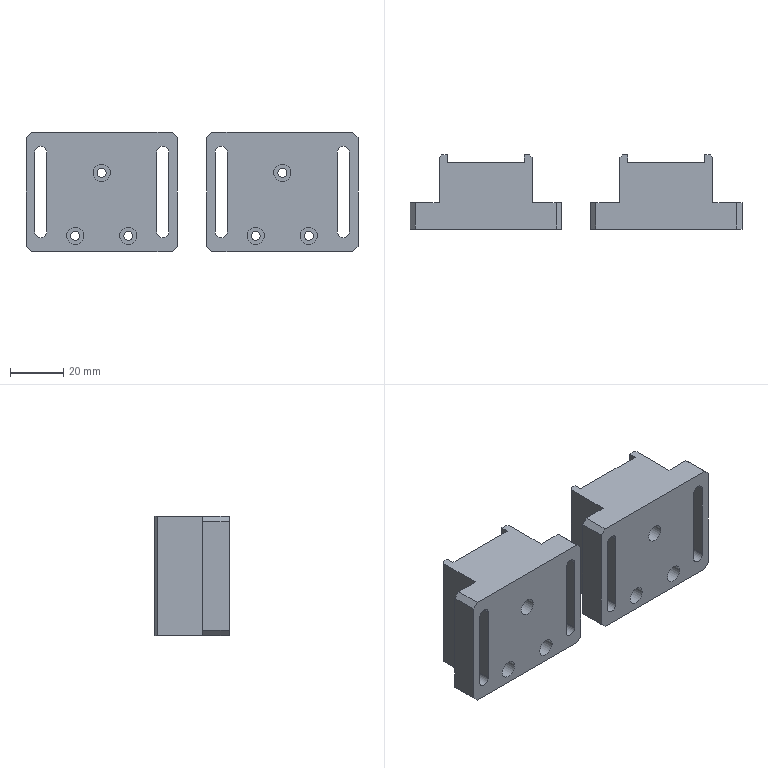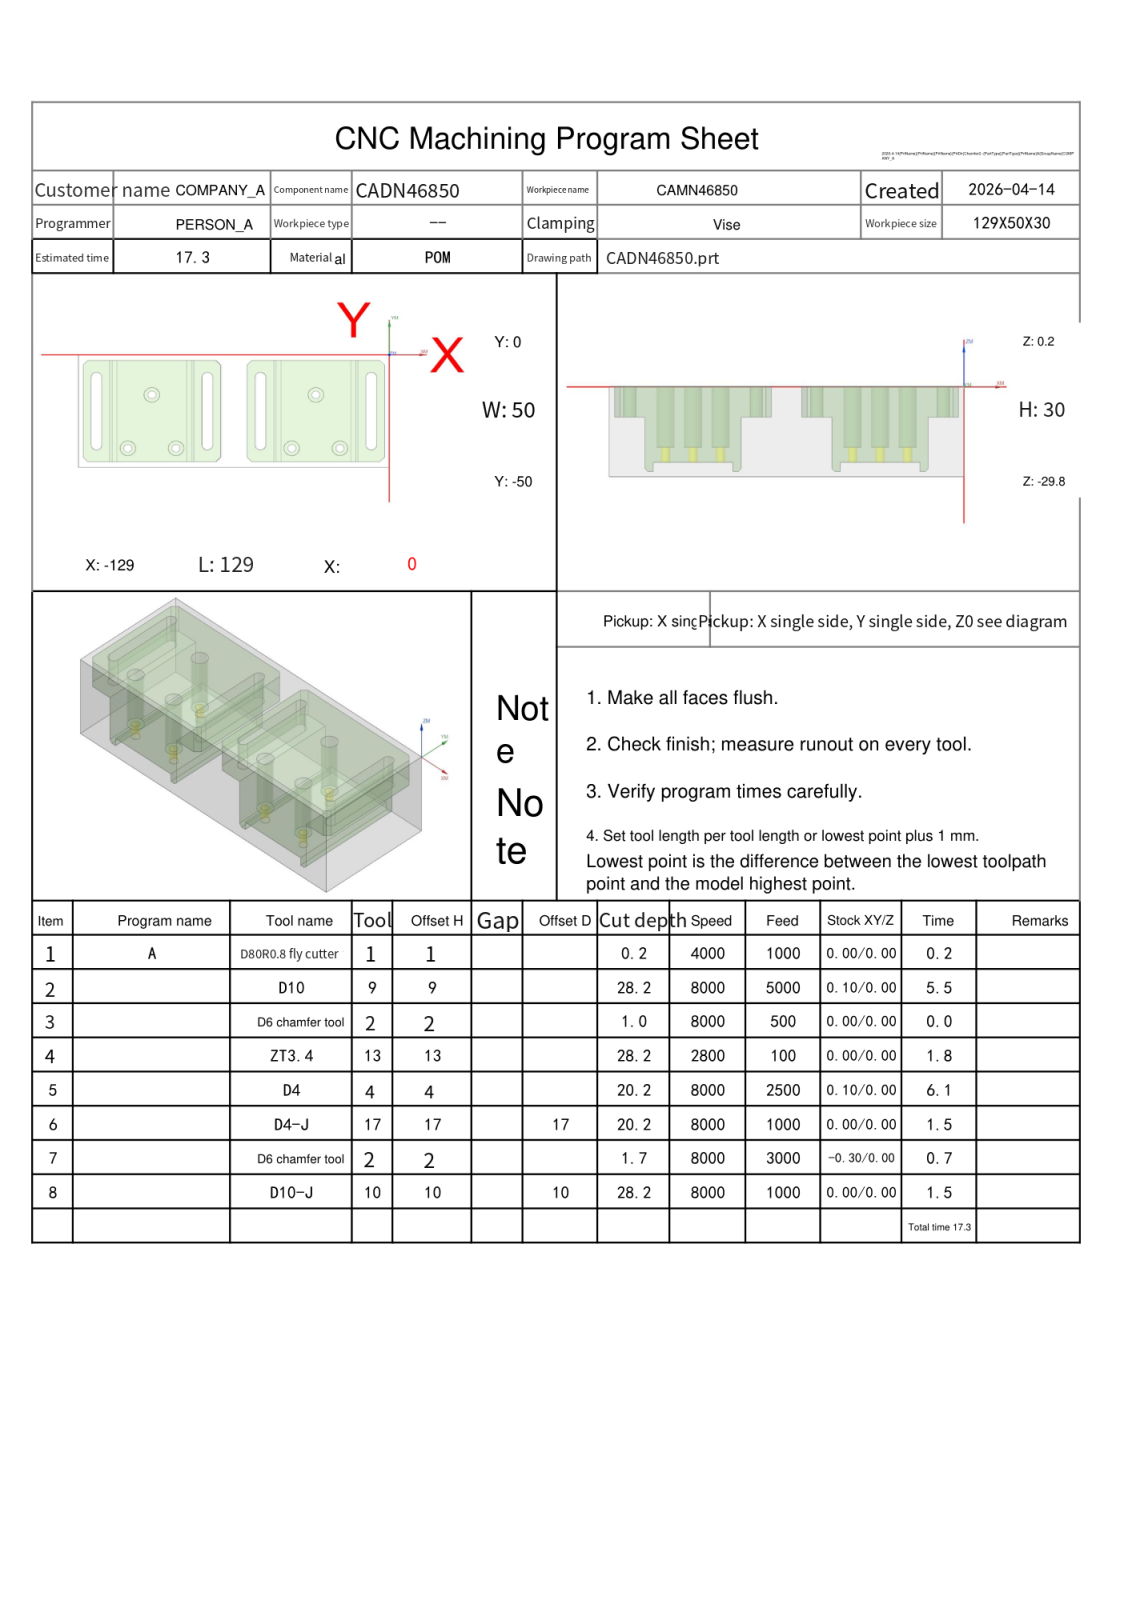NC program | NX | posted by the shop | part box 125 x 28 x 45 mm
Lines 1 to 33 of 4607:
%
O0001
(Machine time: 17.84 MIN)
(===Total Tool:7===)
(T1=D80R0.8 fly cutter D=80.  R=0.8  D-  H01 Z=0.    )
(T9=D10     D=10.  R=0.   D-  H09 Z=-28.  )
(T2=D6 chamfer tool   D=6.   R=0.   D-  H02 Z=-1.5  )
(T13=ZT3.4  D=3.4  DR_a=118 D-  H13 Z=-28.02)
(T4=D4      D=4.   R=0.   D-  H04 Z=-20.  )
(T17=D4-J   D=4.   R=0.   D17 H17 Z=-20.  )
(T10=D10-J  D=10.  R=0.   D10 H10 Z=-28.  )
G80 G90 G17 G49 G40
G91 G28 Z0
M01
N1 T01 M06
(D80R0.8 fly cutter  D=80. R=0.8 H=01 ce=0.00 di=0.00)
G00 G90 G54 X43. Y-25. M03 S4000
G43 H01 Z20.
M08
Z2.
G01 Z0.0 F1000.
X38.
X-167.
X-172.
Z2.
G00 Z20.
G91 G28 Z0.0
M05
M09
G91 G28 Z0.0
M01